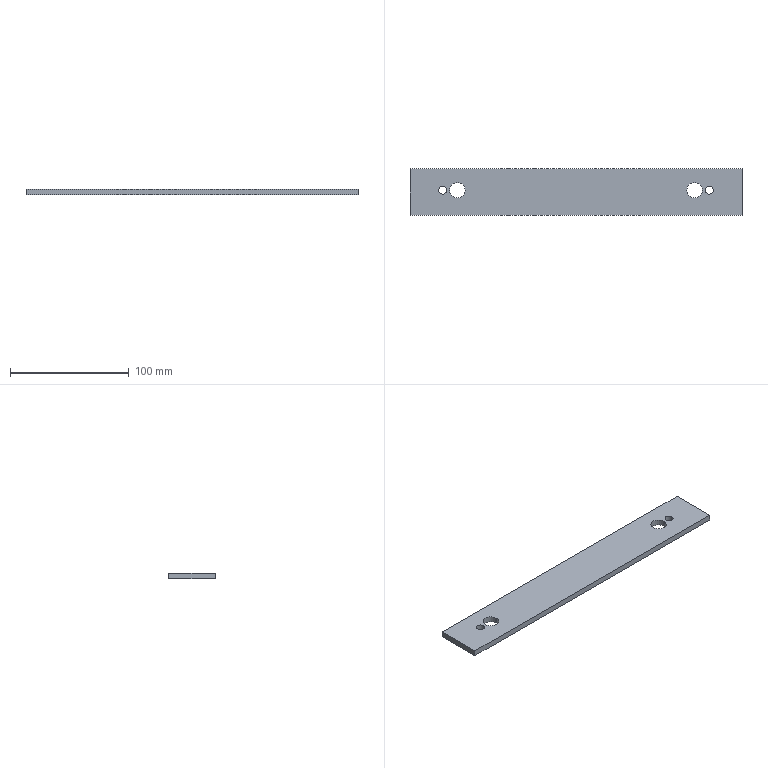Part | STEP file | 44-02-08 Ear Forming Plate A | 1 solid | 14 faces | box 280 x 39 x 5 mm | volume 52910 mm3 | cylinder 8 | plane 6 | commonest cylinder face diameters 6.8 x4 13 x4
STEP:
#1=CARTESIAN_POINT('',(0.,0.,0.));
#2=DIRECTION('',(0.,0.,1.));
#3=DIRECTION('',(1.,0.,0.));
#4=AXIS2_PLACEMENT_3D('',#1,#2,#3);
#5=CARTESIAN_POINT('',(109.1,0.,2.5));
#6=VERTEX_POINT('',#5);
#7=CARTESIAN_POINT('',(109.1,0.,-2.5));
#8=VERTEX_POINT('',#7);
#9=CARTESIAN_POINT('',(109.1,0.,-2.5));
#10=DIRECTION('',(0.,0.,-1.));
#11=VECTOR('',#10,1.);
#12=LINE('',#9,#11);
#13=CARTESIAN_POINT('',(112.5,0.,-2.5));
#14=DIRECTION('',(0.,0.,-1.));
#15=DIRECTION('',(-1.,0.,0.));
#16=AXIS2_PLACEMENT_3D('',#13,#14,#15);
#17=CYLINDRICAL_SURFACE('',#16,3.4);
#18=CARTESIAN_POINT('',(6.283,0.));
#19=DIRECTION('',(0.,1.));
#20=VECTOR('',#19,1.);
#21=LINE('',#18,#20);
#22=(GEOMETRIC_REPRESENTATION_CONTEXT(2)PARAMETRIC_REPRESENTATION_CONTEXT()REPRESENTATION_CONTEXT('',''));
#23=DEFINITIONAL_REPRESENTATION('',(#21),#22);
#24=PCURVE('',#17,#23);
#25=CARTESIAN_POINT('',(112.5,0.,-2.5));
#26=DIRECTION('',(0.,0.,-1.));
#27=DIRECTION('',(-1.,0.,0.));
#28=AXIS2_PLACEMENT_3D('',#25,#26,#27);
#29=CYLINDRICAL_SURFACE('',#28,3.4);
#30=CARTESIAN_POINT('',(0.,0.));
#31=DIRECTION('',(0.,1.));
#32=VECTOR('',#31,1.);
#33=LINE('',#30,#32);
#34=(GEOMETRIC_REPRESENTATION_CONTEXT(2)PARAMETRIC_REPRESENTATION_CONTEXT()REPRESENTATION_CONTEXT('',''));
#35=DEFINITIONAL_REPRESENTATION('',(#33),#34);
#36=PCURVE('',#29,#35);
#37=SURFACE_CURVE('',#12,(#24,#36),.PCURVE_S1.);
#38=EDGE_CURVE('',#6,#8,#37,.T.);
#39=ORIENTED_EDGE('',*,*,#38,.T.);
#40=CARTESIAN_POINT('',(115.9,0.,-2.5));
#41=VERTEX_POINT('',#40);
#42=CARTESIAN_POINT('',(112.5,0.,-2.5));
#43=DIRECTION('',(0.,0.,-1.));
#44=DIRECTION('',(-1.,0.,0.));
#45=AXIS2_PLACEMENT_3D('',#42,#43,#44);
#46=CIRCLE('',#45,3.4);
#47=CARTESIAN_POINT('',(0.,0.));
#48=DIRECTION('',(1.,0.));
#49=VECTOR('',#48,1.);
#50=LINE('',#47,#49);
#51=(GEOMETRIC_REPRESENTATION_CONTEXT(2)PARAMETRIC_REPRESENTATION_CONTEXT()REPRESENTATION_CONTEXT('',''));
#52=DEFINITIONAL_REPRESENTATION('',(#50),#51);
#53=PCURVE('',#17,#52);
#54=CARTESIAN_POINT('',(140.,-18.,-2.5));
#55=DIRECTION('',(0.,0.,1.));
#56=DIRECTION('',(1.,0.,0.));
#57=AXIS2_PLACEMENT_3D('',#54,#55,#56);
#58=PLANE('',#57);
#59=CARTESIAN_POINT('',(-30.9,18.));
#60=CARTESIAN_POINT('',(-30.9,23.889));
#61=CARTESIAN_POINT('',(-25.8,20.944));
#62=CARTESIAN_POINT('',(-20.7,18.));
#63=CARTESIAN_POINT('',(-25.8,15.056));
#64=CARTESIAN_POINT('',(-30.9,12.111));
#65=CARTESIAN_POINT('',(-30.9,18.));
#66=(BOUNDED_CURVE()B_SPLINE_CURVE(2,(#59,#60,#61,#62,#63,#64,#65),.UNSPECIFIED.,.T.,.F.)B_SPLINE_CURVE_WITH_KNOTS((1,2,2,2,2,1),(-2.094,0.,2.094,4.189,6.283,8.378),.UNSPECIFIED.)CURVE()GEOMETRIC_REPRESENTATION_ITEM()RATIONAL_B_SPLINE_CURVE((1.,0.5,1.,0.5,1.,0.5,1.))REPRESENTATION_ITEM(''));
#67=(GEOMETRIC_REPRESENTATION_CONTEXT(2)PARAMETRIC_REPRESENTATION_CONTEXT()REPRESENTATION_CONTEXT('',''));
#68=DEFINITIONAL_REPRESENTATION('',(#66),#67);
#69=PCURVE('',#58,#68);
#70=SURFACE_CURVE('',#46,(#53,#69),.PCURVE_S1.);
#71=EDGE_CURVE('',#41,#8,#70,.T.);
#72=ORIENTED_EDGE('',*,*,#71,.F.);
#73=CARTESIAN_POINT('',(115.9,0.,2.5));
#74=VERTEX_POINT('',#73);
#75=CARTESIAN_POINT('',(115.9,0.,-2.5));
#76=DIRECTION('',(0.,0.,-1.));
#77=VECTOR('',#76,1.);
#78=LINE('',#75,#77);
#79=CARTESIAN_POINT('',(3.142,0.));
#80=DIRECTION('',(0.,1.));
#81=VECTOR('',#80,1.);
#82=LINE('',#79,#81);
#83=(GEOMETRIC_REPRESENTATION_CONTEXT(2)PARAMETRIC_REPRESENTATION_CONTEXT()REPRESENTATION_CONTEXT('',''));
#84=DEFINITIONAL_REPRESENTATION('',(#82),#83);
#85=PCURVE('',#17,#84);
#86=CARTESIAN_POINT('',(3.142,0.));
#87=DIRECTION('',(0.,1.));
#88=VECTOR('',#87,1.);
#89=LINE('',#86,#88);
#90=(GEOMETRIC_REPRESENTATION_CONTEXT(2)PARAMETRIC_REPRESENTATION_CONTEXT()REPRESENTATION_CONTEXT('',''));
#91=DEFINITIONAL_REPRESENTATION('',(#89),#90);
#92=PCURVE('',#29,#91);
#93=SURFACE_CURVE('',#78,(#85,#92),.PCURVE_S1.);
#94=EDGE_CURVE('',#74,#41,#93,.T.);
#95=ORIENTED_EDGE('',*,*,#94,.F.);
#96=CARTESIAN_POINT('',(112.5,0.,2.5));
#97=DIRECTION('',(0.,0.,-1.));
#98=DIRECTION('',(-1.,0.,0.));
#99=AXIS2_PLACEMENT_3D('',#96,#97,#98);
#100=CIRCLE('',#99,3.4);
#101=CARTESIAN_POINT('',(0.,-5.));
#102=DIRECTION('',(1.,0.));
#103=VECTOR('',#102,1.);
#104=LINE('',#101,#103);
#105=(GEOMETRIC_REPRESENTATION_CONTEXT(2)PARAMETRIC_REPRESENTATION_CONTEXT()REPRESENTATION_CONTEXT('',''));
#106=DEFINITIONAL_REPRESENTATION('',(#104),#105);
#107=PCURVE('',#17,#106);
#108=CARTESIAN_POINT('',(140.,-18.,2.5));
#109=DIRECTION('',(0.,0.,1.));
#110=DIRECTION('',(1.,0.,0.));
#111=AXIS2_PLACEMENT_3D('',#108,#109,#110);
#112=PLANE('',#111);
#113=CARTESIAN_POINT('',(-30.9,18.));
#114=CARTESIAN_POINT('',(-30.9,23.889));
#115=CARTESIAN_POINT('',(-25.8,20.944));
#116=CARTESIAN_POINT('',(-20.7,18.));
#117=CARTESIAN_POINT('',(-25.8,15.056));
#118=CARTESIAN_POINT('',(-30.9,12.111));
#119=CARTESIAN_POINT('',(-30.9,18.));
#120=(BOUNDED_CURVE()B_SPLINE_CURVE(2,(#113,#114,#115,#116,#117,#118,#119),.UNSPECIFIED.,.T.,.F.)B_SPLINE_CURVE_WITH_KNOTS((1,2,2,2,2,1),(-2.094,0.,2.094,4.189,6.283,8.378),.UNSPECIFIED.)CURVE()GEOMETRIC_REPRESENTATION_ITEM()RATIONAL_B_SPLINE_CURVE((1.,0.5,1.,0.5,1.,0.5,1.))REPRESENTATION_ITEM(''));
#121=(GEOMETRIC_REPRESENTATION_CONTEXT(2)PARAMETRIC_REPRESENTATION_CONTEXT()REPRESENTATION_CONTEXT('',''));
#122=DEFINITIONAL_REPRESENTATION('',(#120),#121);
#123=PCURVE('',#112,#122);
#124=SURFACE_CURVE('',#100,(#107,#123),.PCURVE_S1.);
#125=EDGE_CURVE('',#74,#6,#124,.T.);
#126=ORIENTED_EDGE('',*,*,#125,.T.);
#127=EDGE_LOOP('',(#39,#72,#95,#126));
#128=FACE_BOUND('',#127,.F.);
#129=ADVANCED_FACE('',(#128),#17,.F.);
#130=CARTESIAN_POINT('',(-115.9,0.,2.5));
#131=VERTEX_POINT('',#130);
#132=CARTESIAN_POINT('',(-115.9,0.,-2.5));
#133=VERTEX_POINT('',#132);
#134=CARTESIAN_POINT('',(-115.9,0.,-2.5));
#135=DIRECTION('',(0.,0.,-1.));
#136=VECTOR('',#135,1.);
#137=LINE('',#134,#136);
#138=CARTESIAN_POINT('',(-112.5,0.,-2.5));
#139=DIRECTION('',(0.,0.,-1.));
#140=DIRECTION('',(-1.,0.,0.));
#141=AXIS2_PLACEMENT_3D('',#138,#139,#140);
#142=CYLINDRICAL_SURFACE('',#141,3.4);
#143=CARTESIAN_POINT('',(6.283,0.));
#144=DIRECTION('',(0.,1.));
#145=VECTOR('',#144,1.);
#146=LINE('',#143,#145);
#147=(GEOMETRIC_REPRESENTATION_CONTEXT(2)PARAMETRIC_REPRESENTATION_CONTEXT()REPRESENTATION_CONTEXT('',''));
#148=DEFINITIONAL_REPRESENTATION('',(#146),#147);
#149=PCURVE('',#142,#148);
#150=CARTESIAN_POINT('',(-112.5,0.,-2.5));
#151=DIRECTION('',(0.,0.,-1.));
#152=DIRECTION('',(-1.,0.,0.));
#153=AXIS2_PLACEMENT_3D('',#150,#151,#152);
#154=CYLINDRICAL_SURFACE('',#153,3.4);
#155=CARTESIAN_POINT('',(0.,0.));
#156=DIRECTION('',(0.,1.));
#157=VECTOR('',#156,1.);
#158=LINE('',#155,#157);
#159=(GEOMETRIC_REPRESENTATION_CONTEXT(2)PARAMETRIC_REPRESENTATION_CONTEXT()REPRESENTATION_CONTEXT('',''));
#160=DEFINITIONAL_REPRESENTATION('',(#158),#159);
#161=PCURVE('',#154,#160);
#162=SURFACE_CURVE('',#137,(#149,#161),.PCURVE_S1.);
#163=EDGE_CURVE('',#131,#133,#162,.T.);
#164=ORIENTED_EDGE('',*,*,#163,.T.);
#165=CARTESIAN_POINT('',(-109.1,0.,-2.5));
#166=VERTEX_POINT('',#165);
#167=CARTESIAN_POINT('',(-112.5,0.,-2.5));
#168=DIRECTION('',(0.,0.,-1.));
#169=DIRECTION('',(-1.,0.,0.));
#170=AXIS2_PLACEMENT_3D('',#167,#168,#169);
#171=CIRCLE('',#170,3.4);
#172=CARTESIAN_POINT('',(0.,0.));
#173=DIRECTION('',(1.,0.));
#174=VECTOR('',#173,1.);
#175=LINE('',#172,#174);
#176=(GEOMETRIC_REPRESENTATION_CONTEXT(2)PARAMETRIC_REPRESENTATION_CONTEXT()REPRESENTATION_CONTEXT('',''));
#177=DEFINITIONAL_REPRESENTATION('',(#175),#176);
#178=PCURVE('',#142,#177);
#179=CARTESIAN_POINT('',(-255.9,18.));
#180=CARTESIAN_POINT('',(-255.9,23.889));
#181=CARTESIAN_POINT('',(-250.8,20.944));
#182=CARTESIAN_POINT('',(-245.7,18.));
#183=CARTESIAN_POINT('',(-250.8,15.056));
#184=CARTESIAN_POINT('',(-255.9,12.111));
#185=CARTESIAN_POINT('',(-255.9,18.));
#186=(BOUNDED_CURVE()B_SPLINE_CURVE(2,(#179,#180,#181,#182,#183,#184,#185),.UNSPECIFIED.,.T.,.F.)B_SPLINE_CURVE_WITH_KNOTS((1,2,2,2,2,1),(-2.094,0.,2.094,4.189,6.283,8.378),.UNSPECIFIED.)CURVE()GEOMETRIC_REPRESENTATION_ITEM()RATIONAL_B_SPLINE_CURVE((1.,0.5,1.,0.5,1.,0.5,1.))REPRESENTATION_ITEM(''));
#187=(GEOMETRIC_REPRESENTATION_CONTEXT(2)PARAMETRIC_REPRESENTATION_CONTEXT()REPRESENTATION_CONTEXT('',''));
#188=DEFINITIONAL_REPRESENTATION('',(#186),#187);
#189=PCURVE('',#58,#188);
#190=SURFACE_CURVE('',#171,(#178,#189),.PCURVE_S1.);
#191=EDGE_CURVE('',#166,#133,#190,.T.);
#192=ORIENTED_EDGE('',*,*,#191,.F.);
#193=CARTESIAN_POINT('',(-109.1,0.,2.5));
#194=VERTEX_POINT('',#193);
#195=CARTESIAN_POINT('',(-109.1,0.,-2.5));
#196=DIRECTION('',(0.,0.,-1.));
#197=VECTOR('',#196,1.);
#198=LINE('',#195,#197);
#199=CARTESIAN_POINT('',(3.142,0.));
#200=DIRECTION('',(0.,1.));
#201=VECTOR('',#200,1.);
#202=LINE('',#199,#201);
#203=(GEOMETRIC_REPRESENTATION_CONTEXT(2)PARAMETRIC_REPRESENTATION_CONTEXT()REPRESENTATION_CONTEXT('',''));
#204=DEFINITIONAL_REPRESENTATION('',(#202),#203);
#205=PCURVE('',#142,#204);
#206=CARTESIAN_POINT('',(3.142,0.));
#207=DIRECTION('',(0.,1.));
#208=VECTOR('',#207,1.);
#209=LINE('',#206,#208);
#210=(GEOMETRIC_REPRESENTATION_CONTEXT(2)PARAMETRIC_REPRESENTATION_CONTEXT()REPRESENTATION_CONTEXT('',''));
#211=DEFINITIONAL_REPRESENTATION('',(#209),#210);
#212=PCURVE('',#154,#211);
#213=SURFACE_CURVE('',#198,(#205,#212),.PCURVE_S1.);
#214=EDGE_CURVE('',#194,#166,#213,.T.);
#215=ORIENTED_EDGE('',*,*,#214,.F.);
#216=CARTESIAN_POINT('',(-112.5,0.,2.5));
#217=DIRECTION('',(0.,0.,-1.));
#218=DIRECTION('',(-1.,0.,0.));
#219=AXIS2_PLACEMENT_3D('',#216,#217,#218);
#220=CIRCLE('',#219,3.4);
#221=CARTESIAN_POINT('',(0.,-5.));
#222=DIRECTION('',(1.,0.));
#223=VECTOR('',#222,1.);
#224=LINE('',#221,#223);
#225=(GEOMETRIC_REPRESENTATION_CONTEXT(2)PARAMETRIC_REPRESENTATION_CONTEXT()REPRESENTATION_CONTEXT('',''));
#226=DEFINITIONAL_REPRESENTATION('',(#224),#225);
#227=PCURVE('',#142,#226);
#228=CARTESIAN_POINT('',(-255.9,18.));
#229=CARTESIAN_POINT('',(-255.9,23.889));
#230=CARTESIAN_POINT('',(-250.8,20.944));
#231=CARTESIAN_POINT('',(-245.7,18.));
#232=CARTESIAN_POINT('',(-250.8,15.056));
#233=CARTESIAN_POINT('',(-255.9,12.111));
#234=CARTESIAN_POINT('',(-255.9,18.));
#235=(BOUNDED_CURVE()B_SPLINE_CURVE(2,(#228,#229,#230,#231,#232,#233,#234),.UNSPECIFIED.,.T.,.F.)B_SPLINE_CURVE_WITH_KNOTS((1,2,2,2,2,1),(-2.094,0.,2.094,4.189,6.283,8.378),.UNSPECIFIED.)CURVE()GEOMETRIC_REPRESENTATION_ITEM()RATIONAL_B_SPLINE_CURVE((1.,0.5,1.,0.5,1.,0.5,1.))REPRESENTATION_ITEM(''));
#236=(GEOMETRIC_REPRESENTATION_CONTEXT(2)PARAMETRIC_REPRESENTATION_CONTEXT()REPRESENTATION_CONTEXT('',''));
#237=DEFINITIONAL_REPRESENTATION('',(#235),#236);
#238=PCURVE('',#112,#237);
#239=SURFACE_CURVE('',#220,(#227,#238),.PCURVE_S1.);
#240=EDGE_CURVE('',#194,#131,#239,.T.);
#241=ORIENTED_EDGE('',*,*,#240,.T.);
#242=EDGE_LOOP('',(#164,#192,#215,#241));
#243=FACE_BOUND('',#242,.F.);
#244=ADVANCED_FACE('',(#243),#142,.F.);
#245=CARTESIAN_POINT('',(106.5,0.,-2.5));
#246=VERTEX_POINT('',#245);
#247=CARTESIAN_POINT('',(106.5,0.,2.5));
#248=VERTEX_POINT('',#247);
#249=CARTESIAN_POINT('',(106.5,0.,-2.5));
#250=DIRECTION('',(0.,0.,1.));
#251=VECTOR('',#250,1.);
#252=LINE('',#249,#251);
#253=CARTESIAN_POINT('',(100.,0.,-2.5));
#254=DIRECTION('',(0.,0.,1.));
#255=DIRECTION('',(1.,0.,0.));
#256=AXIS2_PLACEMENT_3D('',#253,#254,#255);
#257=CYLINDRICAL_SURFACE('',#256,6.5);
#258=CARTESIAN_POINT('',(6.283,0.));
#259=DIRECTION('',(0.,1.));
#260=VECTOR('',#259,1.);
#261=LINE('',#258,#260);
#262=(GEOMETRIC_REPRESENTATION_CONTEXT(2)PARAMETRIC_REPRESENTATION_CONTEXT()REPRESENTATION_CONTEXT('',''));
#263=DEFINITIONAL_REPRESENTATION('',(#261),#262);
#264=PCURVE('',#257,#263);
#265=CARTESIAN_POINT('',(100.,0.,-2.5));
#266=DIRECTION('',(0.,0.,1.));
#267=DIRECTION('',(1.,0.,0.));
#268=AXIS2_PLACEMENT_3D('',#265,#266,#267);
#269=CYLINDRICAL_SURFACE('',#268,6.5);
#270=CARTESIAN_POINT('',(0.,0.));
#271=DIRECTION('',(0.,1.));
#272=VECTOR('',#271,1.);
#273=LINE('',#270,#272);
#274=(GEOMETRIC_REPRESENTATION_CONTEXT(2)PARAMETRIC_REPRESENTATION_CONTEXT()REPRESENTATION_CONTEXT('',''));
#275=DEFINITIONAL_REPRESENTATION('',(#273),#274);
#276=PCURVE('',#269,#275);
#277=SURFACE_CURVE('',#252,(#264,#276),.PCURVE_S1.);
#278=EDGE_CURVE('',#246,#248,#277,.T.);
#279=ORIENTED_EDGE('',*,*,#278,.T.);
#280=CARTESIAN_POINT('',(93.5,0.,2.5));
#281=VERTEX_POINT('',#280);
#282=CARTESIAN_POINT('',(100.,0.,2.5));
#283=DIRECTION('',(0.,0.,1.));
#284=DIRECTION('',(1.,0.,0.));
#285=AXIS2_PLACEMENT_3D('',#282,#283,#284);
#286=CIRCLE('',#285,6.5);
#287=CARTESIAN_POINT('',(0.,5.));
#288=DIRECTION('',(1.,0.));
#289=VECTOR('',#288,1.);
#290=LINE('',#287,#289);
#291=(GEOMETRIC_REPRESENTATION_CONTEXT(2)PARAMETRIC_REPRESENTATION_CONTEXT()REPRESENTATION_CONTEXT('',''));
#292=DEFINITIONAL_REPRESENTATION('',(#290),#291);
#293=PCURVE('',#257,#292);
#294=CARTESIAN_POINT('',(-40.,18.));
#295=DIRECTION('',(1.,0.));
#296=AXIS2_PLACEMENT_2D('',#294,#295);
#297=CIRCLE('',#296,6.5);
#298=(GEOMETRIC_REPRESENTATION_CONTEXT(2)PARAMETRIC_REPRESENTATION_CONTEXT()REPRESENTATION_CONTEXT('',''));
#299=DEFINITIONAL_REPRESENTATION('',(#297),#298);
#300=PCURVE('',#112,#299);
#301=SURFACE_CURVE('',#286,(#293,#300),.PCURVE_S1.);
#302=EDGE_CURVE('',#281,#248,#301,.T.);
#303=ORIENTED_EDGE('',*,*,#302,.F.);
#304=CARTESIAN_POINT('',(93.5,0.,-2.5));
#305=VERTEX_POINT('',#304);
#306=CARTESIAN_POINT('',(93.5,0.,-2.5));
#307=DIRECTION('',(0.,0.,1.));
#308=VECTOR('',#307,1.);
#309=LINE('',#306,#308);
#310=CARTESIAN_POINT('',(3.142,0.));
#311=DIRECTION('',(0.,1.));
#312=VECTOR('',#311,1.);
#313=LINE('',#310,#312);
#314=(GEOMETRIC_REPRESENTATION_CONTEXT(2)PARAMETRIC_REPRESENTATION_CONTEXT()REPRESENTATION_CONTEXT('',''));
#315=DEFINITIONAL_REPRESENTATION('',(#313),#314);
#316=PCURVE('',#257,#315);
#317=CARTESIAN_POINT('',(3.142,0.));
#318=DIRECTION('',(0.,1.));
#319=VECTOR('',#318,1.);
#320=LINE('',#317,#319);
#321=(GEOMETRIC_REPRESENTATION_CONTEXT(2)PARAMETRIC_REPRESENTATION_CONTEXT()REPRESENTATION_CONTEXT('',''));
#322=DEFINITIONAL_REPRESENTATION('',(#320),#321);
#323=PCURVE('',#269,#322);
#324=SURFACE_CURVE('',#309,(#316,#323),.PCURVE_S1.);
#325=EDGE_CURVE('',#305,#281,#324,.T.);
#326=ORIENTED_EDGE('',*,*,#325,.F.);
#327=CARTESIAN_POINT('',(100.,0.,-2.5));
#328=DIRECTION('',(0.,0.,1.));
#329=DIRECTION('',(1.,0.,0.));
#330=AXIS2_PLACEMENT_3D('',#327,#328,#329);
#331=CIRCLE('',#330,6.5);
#332=CARTESIAN_POINT('',(0.,0.));
#333=DIRECTION('',(1.,0.));
#334=VECTOR('',#333,1.);
#335=LINE('',#332,#334);
#336=(GEOMETRIC_REPRESENTATION_CONTEXT(2)PARAMETRIC_REPRESENTATION_CONTEXT()REPRESENTATION_CONTEXT('',''));
#337=DEFINITIONAL_REPRESENTATION('',(#335),#336);
#338=PCURVE('',#257,#337);
#339=CARTESIAN_POINT('',(-40.,18.));
#340=DIRECTION('',(1.,0.));
#341=AXIS2_PLACEMENT_2D('',#339,#340);
#342=CIRCLE('',#341,6.5);
#343=(GEOMETRIC_REPRESENTATION_CONTEXT(2)PARAMETRIC_REPRESENTATION_CONTEXT()REPRESENTATION_CONTEXT('',''));
#344=DEFINITIONAL_REPRESENTATION('',(#342),#343);
#345=PCURVE('',#58,#344);
#346=SURFACE_CURVE('',#331,(#338,#345),.PCURVE_S1.);
#347=EDGE_CURVE('',#305,#246,#346,.T.);
#348=ORIENTED_EDGE('',*,*,#347,.T.);
#349=EDGE_LOOP('',(#279,#303,#326,#348));
#350=FACE_BOUND('',#349,.F.);
#351=ADVANCED_FACE('',(#350),#257,.F.);
#352=CARTESIAN_POINT('',(-93.5,0.,-2.5));
#353=VERTEX_POINT('',#352);
#354=CARTESIAN_POINT('',(-93.5,0.,2.5));
#355=VERTEX_POINT('',#354);
#356=CARTESIAN_POINT('',(-93.5,0.,-2.5));
#357=DIRECTION('',(0.,0.,1.));
#358=VECTOR('',#357,1.);
#359=LINE('',#356,#358);
#360=CARTESIAN_POINT('',(-100.,0.,-2.5));
#361=DIRECTION('',(0.,0.,1.));
#362=DIRECTION('',(1.,0.,0.));
#363=AXIS2_PLACEMENT_3D('',#360,#361,#362);
#364=CYLINDRICAL_SURFACE('',#363,6.5);
#365=CARTESIAN_POINT('',(6.283,0.));
#366=DIRECTION('',(0.,1.));
#367=VECTOR('',#366,1.);
#368=LINE('',#365,#367);
#369=(GEOMETRIC_REPRESENTATION_CONTEXT(2)PARAMETRIC_REPRESENTATION_CONTEXT()REPRESENTATION_CONTEXT('',''));
#370=DEFINITIONAL_REPRESENTATION('',(#368),#369);
#371=PCURVE('',#364,#370);
#372=CARTESIAN_POINT('',(-100.,0.,-2.5));
#373=DIRECTION('',(0.,0.,1.));
#374=DIRECTION('',(1.,0.,0.));
#375=AXIS2_PLACEMENT_3D('',#372,#373,#374);
#376=CYLINDRICAL_SURFACE('',#375,6.5);
#377=CARTESIAN_POINT('',(0.,0.));
#378=DIRECTION('',(0.,1.));
#379=VECTOR('',#378,1.);
#380=LINE('',#377,#379);
#381=(GEOMETRIC_REPRESENTATION_CONTEXT(2)PARAMETRIC_REPRESENTATION_CONTEXT()REPRESENTATION_CONTEXT('',''));
#382=DEFINITIONAL_REPRESENTATION('',(#380),#381);
#383=PCURVE('',#376,#382);
#384=SURFACE_CURVE('',#359,(#371,#383),.PCURVE_S1.);
#385=EDGE_CURVE('',#353,#355,#384,.T.);
#386=ORIENTED_EDGE('',*,*,#385,.T.);
#387=CARTESIAN_POINT('',(-106.5,0.,2.5));
#388=VERTEX_POINT('',#387);
#389=CARTESIAN_POINT('',(-100.,0.,2.5));
#390=DIRECTION('',(0.,0.,1.));
#391=DIRECTION('',(1.,0.,0.));
#392=AXIS2_PLACEMENT_3D('',#389,#390,#391);
#393=CIRCLE('',#392,6.5);
#394=CARTESIAN_POINT('',(0.,5.));
#395=DIRECTION('',(1.,0.));
#396=VECTOR('',#395,1.);
#397=LINE('',#394,#396);
#398=(GEOMETRIC_REPRESENTATION_CONTEXT(2)PARAMETRIC_REPRESENTATION_CONTEXT()REPRESENTATION_CONTEXT('',''));
#399=DEFINITIONAL_REPRESENTATION('',(#397),#398);
#400=PCURVE('',#364,#399);
#401=CARTESIAN_POINT('',(-240.,18.));
#402=DIRECTION('',(1.,0.));
#403=AXIS2_PLACEMENT_2D('',#401,#402);
#404=CIRCLE('',#403,6.5);
#405=(GEOMETRIC_REPRESENTATION_CONTEXT(2)PARAMETRIC_REPRESENTATION_CONTEXT()REPRESENTATION_CONTEXT('',''));
#406=DEFINITIONAL_REPRESENTATION('',(#404),#405);
#407=PCURVE('',#112,#406);
#408=SURFACE_CURVE('',#393,(#400,#407),.PCURVE_S1.);
#409=EDGE_CURVE('',#388,#355,#408,.T.);
#410=ORIENTED_EDGE('',*,*,#409,.F.);
#411=CARTESIAN_POINT('',(-106.5,0.,-2.5));
#412=VERTEX_POINT('',#411);
#413=CARTESIAN_POINT('',(-106.5,0.,-2.5));
#414=DIRECTION('',(0.,0.,1.));
#415=VECTOR('',#414,1.);
#416=LINE('',#413,#415);
#417=CARTESIAN_POINT('',(3.142,0.));
#418=DIRECTION('',(0.,1.));
#419=VECTOR('',#418,1.);
#420=LINE('',#417,#419);
#421=(GEOMETRIC_REPRESENTATION_CONTEXT(2)PARAMETRIC_REPRESENTATION_CONTEXT()REPRESENTATION_CONTEXT('',''));
#422=DEFINITIONAL_REPRESENTATION('',(#420),#421);
#423=PCURVE('',#364,#422);
#424=CARTESIAN_POINT('',(3.142,0.));
#425=DIRECTION('',(0.,1.));
#426=VECTOR('',#425,1.);
#427=LINE('',#424,#426);
#428=(GEOMETRIC_REPRESENTATION_CONTEXT(2)PARAMETRIC_REPRESENTATION_CONTEXT()REPRESENTATION_CONTEXT('',''));
#429=DEFINITIONAL_REPRESENTATION('',(#427),#428);
#430=PCURVE('',#376,#429);
#431=SURFACE_CURVE('',#416,(#423,#430),.PCURVE_S1.);
#432=EDGE_CURVE('',#412,#388,#431,.T.);
#433=ORIENTED_EDGE('',*,*,#432,.F.);
#434=CARTESIAN_POINT('',(-100.,0.,-2.5));
#435=DIRECTION('',(0.,0.,1.));
#436=DIRECTION('',(1.,0.,0.));
#437=AXIS2_PLACEMENT_3D('',#434,#435,#436);
#438=CIRCLE('',#437,6.5);
#439=CARTESIAN_POINT('',(0.,0.));
#440=DIRECTION('',(1.,0.));
#441=VECTOR('',#440,1.);
#442=LINE('',#439,#441);
#443=(GEOMETRIC_REPRESENTATION_CONTEXT(2)PARAMETRIC_REPRESENTATION_CONTEXT()REPRESENTATION_CONTEXT('',''));
#444=DEFINITIONAL_REPRESENTATION('',(#442),#443);
#445=PCURVE('',#364,#444);
#446=CARTESIAN_POINT('',(-240.,18.));
#447=DIRECTION('',(1.,0.));
#448=AXIS2_PLACEMENT_2D('',#446,#447);
#449=CIRCLE('',#448,6.5);
#450=(GEOMETRIC_REPRESENTATION_CONTEXT(2)PARAMETRIC_REPRESENTATION_CONTEXT()REPRESENTATION_CONTEXT('',''));
#451=DEFINITIONAL_REPRESENTATION('',(#449),#450);
#452=PCURVE('',#58,#451);
#453=SURFACE_CURVE('',#438,(#445,#452),.PCURVE_S1.);
#454=EDGE_CURVE('',#412,#353,#453,.T.);
#455=ORIENTED_EDGE('',*,*,#454,.T.);
#456=EDGE_LOOP('',(#386,#410,#433,#455));
#457=FACE_BOUND('',#456,.F.);
#458=ADVANCED_FACE('',(#457),#364,.F.);
#459=CARTESIAN_POINT('',(112.5,0.,2.5));
#460=DIRECTION('',(0.,0.,-1.));
#461=DIRECTION('',(-1.,0.,0.));
#462=AXIS2_PLACEMENT_3D('',#459,#460,#461);
#463=CIRCLE('',#462,3.4);
#464=CARTESIAN_POINT('',(-30.9,18.));
#465=CARTESIAN_POINT('',(-30.9,23.889));
#466=CARTESIAN_POINT('',(-25.8,20.944));
#467=CARTESIAN_POINT('',(-20.7,18.));
#468=CARTESIAN_POINT('',(-25.8,15.056));
#469=CARTESIAN_POINT('',(-30.9,12.111));
#470=CARTESIAN_POINT('',(-30.9,18.));
#471=(BOUNDED_CURVE()B_SPLINE_CURVE(2,(#464,#465,#466,#467,#468,#469,#470),.UNSPECIFIED.,.T.,.F.)B_SPLINE_CURVE_WITH_KNOTS((1,2,2,2,2,1),(-2.094,0.,2.094,4.189,6.283,8.378),.UNSPECIFIED.)CURVE()GEOMETRIC_REPRESENTATION_ITEM()RATIONAL_B_SPLINE_CURVE((1.,0.5,1.,0.5,1.,0.5,1.))REPRESENTATION_ITEM(''));
#472=(GEOMETRIC_REPRESENTATION_CONTEXT(2)PARAMETRIC_REPRESENTATION_CONTEXT()REPRESENTATION_CONTEXT('',''));
#473=DEFINITIONAL_REPRESENTATION('',(#471),#472);
#474=PCURVE('',#112,#473);
#475=CARTESIAN_POINT('',(0.,-5.));
#476=DIRECTION('',(1.,0.));
#477=VECTOR('',#476,1.);
#478=LINE('',#475,#477);
#479=(GEOMETRIC_REPRESENTATION_CONTEXT(2)PARAMETRIC_REPRESENTATION_CONTEXT()REPRESENTATION_CONTEXT('',''));
#480=DEFINITIONAL_REPRESENTATION('',(#478),#479);
#481=PCURVE('',#29,#480);
#482=SURFACE_CURVE('',#463,(#474,#481),.PCURVE_S1.);
#483=EDGE_CURVE('',#6,#74,#482,.T.);
#484=ORIENTED_EDGE('',*,*,#483,.T.);
#485=ORIENTED_EDGE('',*,*,#125,.T.);
#486=EDGE_LOOP('',(#484,#485));
#487=FACE_BOUND('',#486,.T.);
#488=CARTESIAN_POINT('',(140.,-21.,2.5));
#489=VERTEX_POINT('',#488);
#490=CARTESIAN_POINT('',(140.,18.,2.5));
#491=VERTEX_POINT('',#490);
#492=CARTESIAN_POINT('',(140.,18.,2.5));
#493=DIRECTION('',(0.,1.,0.));
#494=VECTOR('',#493,1.);
#495=LINE('',#492,#494);
#496=CARTESIAN_POINT('',(0.,36.));
#497=DIRECTION('',(0.,1.));
#498=VECTOR('',#497,1.);
#499=LINE('',#496,#498);
#500=(GEOMETRIC_REPRESENTATION_CONTEXT(2)PARAMETRIC_REPRESENTATION_CONTEXT()REPRESENTATION_CONTEXT('',''));
#501=DEFINITIONAL_REPRESENTATION('',(#499),#500);
#502=PCURVE('',#112,#501);
#503=CARTESIAN_POINT('',(140.,18.,2.5));
#504=DIRECTION('',(-1.,0.,0.));
#505=DIRECTION('',(0.,0.,1.));
#506=AXIS2_PLACEMENT_3D('',#503,#504,#505);
#507=PLANE('',#506);
#508=CARTESIAN_POINT('',(0.,0.));
#509=DIRECTION('',(0.,1.));
#510=VECTOR('',#509,1.);
#511=LINE('',#508,#510);
#512=(GEOMETRIC_REPRESENTATION_CONTEXT(2)PARAMETRIC_REPRESENTATION_CONTEXT()REPRESENTATION_CONTEXT('',''));
#513=DEFINITIONAL_REPRESENTATION('',(#511),#512);
#514=PCURVE('',#507,#513);
#515=SURFACE_CURVE('',#495,(#502,#514),.PCURVE_S1.);
#516=EDGE_CURVE('',#489,#491,#515,.T.);
#517=ORIENTED_EDGE('',*,*,#516,.T.);
#518=CARTESIAN_POINT('',(-140.,18.,2.5));
#519=VERTEX_POINT('',#518);
#520=CARTESIAN_POINT('',(-140.,18.,2.5));
#521=DIRECTION('',(-1.,0.,0.));
#522=VECTOR('',#521,1.);
#523=LINE('',#520,#522);
#524=CARTESIAN_POINT('',(-280.,36.));
#525=DIRECTION('',(-1.,0.));
#526=VECTOR('',#525,1.);
#527=LINE('',#524,#526);
#528=(GEOMETRIC_REPRESENTATION_CONTEXT(2)PARAMETRIC_REPRESENTATION_CONTEXT()REPRESENTATION_CONTEXT('',''));
#529=DEFINITIONAL_REPRESENTATION('',(#527),#528);
#530=PCURVE('',#112,#529);
#531=CARTESIAN_POINT('',(-140.,18.,2.5));
#532=DIRECTION('',(0.,-1.,0.));
#533=DIRECTION('',(0.,0.,-1.));
#534=AXIS2_PLACEMENT_3D('',#531,#532,#533);
#535=PLANE('',#534);
#536=CARTESIAN_POINT('',(0.,0.));
#537=DIRECTION('',(0.,-1.));
#538=VECTOR('',#537,1.);
#539=LINE('',#536,#538);
#540=(GEOMETRIC_REPRESENTATION_CONTEXT(2)PARAMETRIC_REPRESENTATION_CONTEXT()REPRESENTATION_CONTEXT('',''));
#541=DEFINITIONAL_REPRESENTATION('',(#539),#540);
#542=PCURVE('',#535,#541);
#543=SURFACE_CURVE('',#523,(#530,#542),.PCURVE_S1.);
#544=EDGE_CURVE('',#491,#519,#543,.T.);
#545=ORIENTED_EDGE('',*,*,#544,.T.);
#546=CARTESIAN_POINT('',(-140.,-21.,2.5));
#547=VERTEX_POINT('',#546);
#548=CARTESIAN_POINT('',(-140.,18.,2.5));
#549=DIRECTION('',(0.,-1.,0.));
#550=VECTOR('',#549,1.);
#551=LINE('',#548,#550);
#552=CARTESIAN_POINT('',(-280.,36.));
#553=DIRECTION('',(0.,-1.));
#554=VECTOR('',#553,1.);
#555=LINE('',#552,#554);
#556=(GEOMETRIC_REPRESENTATION_CONTEXT(2)PARAMETRIC_REPRESENTATION_CONTEXT()REPRESENTATION_CONTEXT('',''));
#557=DEFINITIONAL_REPRESENTATION('',(#555),#556);
#558=PCURVE('',#112,#557);
#559=CARTESIAN_POINT('',(-140.,18.,2.5));
#560=DIRECTION('',(1.,0.,0.));
#561=DIRECTION('',(0.,0.,-1.));
#562=AXIS2_PLACEMENT_3D('',#559,#560,#561);
#563=PLANE('',#562);
#564=CARTESIAN_POINT('',(0.,0.));
#565=DIRECTION('',(0.,-1.));
#566=VECTOR('',#565,1.);
#567=LINE('',#564,#566);
#568=(GEOMETRIC_REPRESENTATION_CONTEXT(2)PARAMETRIC_REPRESENTATION_CONTEXT()REPRESENTATION_CONTEXT('',''));
#569=DEFINITIONAL_REPRESENTATION('',(#567),#568);
#570=PCURVE('',#563,#569);
#571=SURFACE_CURVE('',#551,(#558,#570),.PCURVE_S1.);
#572=EDGE_CURVE('',#519,#547,#571,.T.);
#573=ORIENTED_EDGE('',*,*,#572,.T.);
#574=CARTESIAN_POINT('',(-140.,-21.,2.5));
#575=DIRECTION('',(1.,0.,0.));
#576=VECTOR('',#575,1.);
#577=LINE('',#574,#576);
#578=CARTESIAN_POINT('',(-280.,-3.));
#579=DIRECTION('',(1.,0.));
#580=VECTOR('',#579,1.);
#581=LINE('',#578,#580);
#582=(GEOMETRIC_REPRESENTATION_CONTEXT(2)PARAMETRIC_REPRESENTATION_CONTEXT()REPRESENTATION_CONTEXT('',''));
#583=DEFINITIONAL_REPRESENTATION('',(#581),#582);
#584=PCURVE('',#112,#583);
#585=CARTESIAN_POINT('',(-140.,-21.,2.5));
#586=DIRECTION('',(0.,1.,0.));
#587=DIRECTION('',(0.,0.,1.));
#588=AXIS2_PLACEMENT_3D('',#585,#586,#587);
#589=PLANE('',#588);
#590=CARTESIAN_POINT('',(0.,0.));
#591=DIRECTION('',(0.,1.));
#592=VECTOR('',#591,1.);
#593=LINE('',#590,#592);
#594=(GEOMETRIC_REPRESENTATION_CONTEXT(2)PARAMETRIC_REPRESENTATION_CONTEXT()REPRESENTATION_CONTEXT('',''));
#595=DEFINITIONAL_REPRESENTATION('',(#593),#594);
#596=PCURVE('',#589,#595);
#597=SURFACE_CURVE('',#577,(#584,#596),.PCURVE_S1.);
#598=EDGE_CURVE('',#547,#489,#597,.T.);
#599=ORIENTED_EDGE('',*,*,#598,.T.);
#600=EDGE_LOOP('',(#517,#545,#573,#599));
#601=FACE_BOUND('',#600,.T.);
#602=CARTESIAN_POINT('',(-100.,0.,2.5));
#603=DIRECTION('',(0.,0.,1.));
#604=DIRECTION('',(1.,0.,0.));
#605=AXIS2_PLACEMENT_3D('',#602,#603,#604);
#606=CIRCLE('',#605,6.5);
#607=CARTESIAN_POINT('',(-240.,18.));
#608=DIRECTION('',(1.,0.));
#609=AXIS2_PLACEMENT_2D('',#607,#608);
#610=CIRCLE('',#609,6.5);
#611=(GEOMETRIC_REPRESENTATION_CONTEXT(2)PARAMETRIC_REPRESENTATION_CONTEXT()REPRESENTATION_CONTEXT('',''));
#612=DEFINITIONAL_REPRESENTATION('',(#610),#611);
#613=PCURVE('',#112,#612);
#614=CARTESIAN_POINT('',(0.,5.));
#615=DIRECTION('',(1.,0.));
#616=VECTOR('',#615,1.);
#617=LINE('',#614,#616);
#618=(GEOMETRIC_REPRESENTATION_CONTEXT(2)PARAMETRIC_REPRESENTATION_CONTEXT()REPRESENTATION_CONTEXT('',''));
#619=DEFINITIONAL_REPRESENTATION('',(#617),#618);
#620=PCURVE('',#376,#619);
#621=SURFACE_CURVE('',#606,(#613,#620),.PCURVE_S1.);
#622=EDGE_CURVE('',#355,#388,#621,.T.);
#623=ORIENTED_EDGE('',*,*,#622,.F.);
#624=ORIENTED_EDGE('',*,*,#409,.F.);
#625=EDGE_LOOP('',(#623,#624));
#626=FACE_BOUND('',#625,.T.);
#627=CARTESIAN_POINT('',(100.,0.,2.5));
#628=DIRECTION('',(0.,0.,1.));
#629=DIRECTION('',(1.,0.,0.));
#630=AXIS2_PLACEMENT_3D('',#627,#628,#629);
#631=CIRCLE('',#630,6.5);
#632=CARTESIAN_POINT('',(-40.,18.));
#633=DIRECTION('',(1.,0.));
#634=AXIS2_PLACEMENT_2D('',#632,#633);
#635=CIRCLE('',#634,6.5);
#636=(GEOMETRIC_REPRESENTATION_CONTEXT(2)PARAMETRIC_REPRESENTATION_CONTEXT()REPRESENTATION_CONTEXT('',''));
#637=DEFINITIONAL_REPRESENTATION('',(#635),#636);
#638=PCURVE('',#112,#637);
#639=CARTESIAN_POINT('',(0.,5.));
#640=DIRECTION('',(1.,0.));
#641=VECTOR('',#640,1.);
#642=LINE('',#639,#641);
#643=(GEOMETRIC_REPRESENTATION_CONTEXT(2)PARAMETRIC_REPRESENTATION_CONTEXT()REPRESENTATION_CONTEXT('',''));
#644=DEFINITIONAL_REPRESENTATION('',(#642),#643);
#645=PCURVE('',#269,#644);
#646=SURFACE_CURVE('',#631,(#638,#645),.PCURVE_S1.);
#647=EDGE_CURVE('',#248,#281,#646,.T.);
#648=ORIENTED_EDGE('',*,*,#647,.F.);
#649=ORIENTED_EDGE('',*,*,#302,.F.);
#650=EDGE_LOOP('',(#648,#649));
#651=FACE_BOUND('',#650,.T.);
#652=CARTESIAN_POINT('',(-112.5,0.,2.5));
#653=DIRECTION('',(0.,0.,-1.));
#654=DIRECTION('',(-1.,0.,0.));
#655=AXIS2_PLACEMENT_3D('',#652,#653,#654);
#656=CIRCLE('',#655,3.4);
#657=CARTESIAN_POINT('',(-255.9,18.));
#658=CARTESIAN_POINT('',(-255.9,23.889));
#659=CARTESIAN_POINT('',(-250.8,20.944));
#660=CARTESIAN_POINT('',(-245.7,18.));
#661=CARTESIAN_POINT('',(-250.8,15.056));
#662=CARTESIAN_POINT('',(-255.9,12.111));
#663=CARTESIAN_POINT('',(-255.9,18.));
#664=(BOUNDED_CURVE()B_SPLINE_CURVE(2,(#657,#658,#659,#660,#661,#662,#663),.UNSPECIFIED.,.T.,.F.)B_SPLINE_CURVE_WITH_KNOTS((1,2,2,2,2,1),(-2.094,0.,2.094,4.189,6.283,8.378),.UNSPECIFIED.)CURVE()GEOMETRIC_REPRESENTATION_ITEM()RATIONAL_B_SPLINE_CURVE((1.,0.5,1.,0.5,1.,0.5,1.))REPRESENTATION_ITEM(''));
#665=(GEOMETRIC_REPRESENTATION_CONTEXT(2)PARAMETRIC_REPRESENTATION_CONTEXT()REPRESENTATION_CONTEXT('',''));
#666=DEFINITIONAL_REPRESENTATION('',(#664),#665);
#667=PCURVE('',#112,#666);
#668=CARTESIAN_POINT('',(0.,-5.));
#669=DIRECTION('',(1.,0.));
#670=VECTOR('',#669,1.);
#671=LINE('',#668,#670);
#672=(GEOMETRIC_REPRESENTATION_CONTEXT(2)PARAMETRIC_REPRESENTATION_CONTEXT()REPRESENTATION_CONTEXT('',''));
#673=DEFINITIONAL_REPRESENTATION('',(#671),#672);
#674=PCURVE('',#154,#673);
#675=SURFACE_CURVE('',#656,(#667,#674),.PCURVE_S1.);
#676=EDGE_CURVE('',#131,#194,#675,.T.);
#677=ORIENTED_EDGE('',*,*,#676,.T.);
#678=ORIENTED_EDGE('',*,*,#240,.T.);
#679=EDGE_LOOP('',(#677,#678));
#680=FACE_BOUND('',#679,.T.);
#681=ADVANCED_FACE('',(#487,#601,#626,#651,#680),#112,.T.);
#682=CARTESIAN_POINT('',(140.,-21.,-2.5));
#683=VERTEX_POINT('',#682);
#684=CARTESIAN_POINT('',(140.,18.,-2.5));
#685=VERTEX_POINT('',#684);
#686=CARTESIAN_POINT('',(140.,18.,-2.5));
#687=DIRECTION('',(0.,1.,0.));
#688=VECTOR('',#687,1.);
#689=LINE('',#686,#688);
#690=CARTESIAN_POINT('',(-5.,0.));
#691=DIRECTION('',(0.,1.));
#692=VECTOR('',#691,1.);
#693=LINE('',#690,#692);
#694=(GEOMETRIC_REPRESENTATION_CONTEXT(2)PARAMETRIC_REPRESENTATION_CONTEXT()REPRESENTATION_CONTEXT('',''));
#695=DEFINITIONAL_REPRESENTATION('',(#693),#694);
#696=PCURVE('',#507,#695);
#697=CARTESIAN_POINT('',(0.,36.));
#698=DIRECTION('',(0.,1.));
#699=VECTOR('',#698,1.);
#700=LINE('',#697,#699);
#701=(GEOMETRIC_REPRESENTATION_CONTEXT(2)PARAMETRIC_REPRESENTATION_CONTEXT()REPRESENTATION_CONTEXT('',''));
#702=DEFINITIONAL_REPRESENTATION('',(#700),#701);
#703=PCURVE('',#58,#702);
#704=SURFACE_CURVE('',#689,(#696,#703),.PCURVE_S1.);
#705=EDGE_CURVE('',#683,#685,#704,.T.);
#706=ORIENTED_EDGE('',*,*,#705,.T.);
#707=CARTESIAN_POINT('',(140.,18.,2.5));
#708=DIRECTION('',(0.,0.,-1.));
#709=VECTOR('',#708,1.);
#710=LINE('',#707,#709);
#711=CARTESIAN_POINT('',(0.,0.));
#712=DIRECTION('',(-1.,0.));
#713=VECTOR('',#712,1.);
#714=LINE('',#711,#713);
#715=(GEOMETRIC_REPRESENTATION_CONTEXT(2)PARAMETRIC_REPRESENTATION_CONTEXT()REPRESENTATION_CONTEXT('',''));
#716=DEFINITIONAL_REPRESENTATION('',(#714),#715);
#717=PCURVE('',#507,#716);
#718=CARTESIAN_POINT('',(0.,280.));
#719=DIRECTION('',(1.,0.));
#720=VECTOR('',#719,1.);
#721=LINE('',#718,#720);
#722=(GEOMETRIC_REPRESENTATION_CONTEXT(2)PARAMETRIC_REPRESENTATION_CONTEXT()REPRESENTATION_CONTEXT('',''));
#723=DEFINITIONAL_REPRESENTATION('',(#721),#722);
#724=PCURVE('',#535,#723);
#725=SURFACE_CURVE('',#710,(#717,#724),.PCURVE_S1.);
#726=EDGE_CURVE('',#491,#685,#725,.T.);
#727=ORIENTED_EDGE('',*,*,#726,.F.);
#728=ORIENTED_EDGE('',*,*,#516,.F.);
#729=CARTESIAN_POINT('',(140.,-21.,-2.5));
#730=DIRECTION('',(0.,0.,-1.));
#731=VECTOR('',#730,1.);
#732=LINE('',#729,#731);
#733=CARTESIAN_POINT('',(-5.,-39.));
#734=DIRECTION('',(-1.,0.));
#735=VECTOR('',#734,1.);
#736=LINE('',#733,#735);
#737=(GEOMETRIC_REPRESENTATION_CONTEXT(2)PARAMETRIC_REPRESENTATION_CONTEXT()REPRESENTATION_CONTEXT('',''));
#738=DEFINITIONAL_REPRESENTATION('',(#736),#737);
#739=PCURVE('',#507,#738);
#740=CARTESIAN_POINT('',(-5.,280.));
#741=DIRECTION('',(-1.,0.));
#742=VECTOR('',#741,1.);
#743=LINE('',#740,#742);
#744=(GEOMETRIC_REPRESENTATION_CONTEXT(2)PARAMETRIC_REPRESENTATION_CONTEXT()REPRESENTATION_CONTEXT('',''));
#745=DEFINITIONAL_REPRESENTATION('',(#743),#744);
#746=PCURVE('',#589,#745);
#747=SURFACE_CURVE('',#732,(#739,#746),.PCURVE_S1.);
#748=EDGE_CURVE('',#489,#683,#747,.T.);
#749=ORIENTED_EDGE('',*,*,#748,.T.);
#750=EDGE_LOOP('',(#706,#727,#728,#749));
#751=FACE_BOUND('',#750,.T.);
#752=ADVANCED_FACE('',(#751),#507,.F.);
#753=CARTESIAN_POINT('',(-140.,18.,-2.5));
#754=VERTEX_POINT('',#753);
#755=CARTESIAN_POINT('',(-140.,18.,-2.5));
#756=DIRECTION('',(-1.,0.,0.));
#757=VECTOR('',#756,1.);
#758=LINE('',#755,#757);
#759=CARTESIAN_POINT('',(5.,0.));
#760=DIRECTION('',(0.,-1.));
#761=VECTOR('',#760,1.);
#762=LINE('',#759,#761);
#763=(GEOMETRIC_REPRESENTATION_CONTEXT(2)PARAMETRIC_REPRESENTATION_CONTEXT()REPRESENTATION_CONTEXT('',''));
#764=DEFINITIONAL_REPRESENTATION('',(#762),#763);
#765=PCURVE('',#535,#764);
#766=CARTESIAN_POINT('',(-280.,36.));
#767=DIRECTION('',(-1.,0.));
#768=VECTOR('',#767,1.);
#769=LINE('',#766,#768);
#770=(GEOMETRIC_REPRESENTATION_CONTEXT(2)PARAMETRIC_REPRESENTATION_CONTEXT()REPRESENTATION_CONTEXT('',''));
#771=DEFINITIONAL_REPRESENTATION('',(#769),#770);
#772=PCURVE('',#58,#771);
#773=SURFACE_CURVE('',#758,(#765,#772),.PCURVE_S1.);
#774=EDGE_CURVE('',#685,#754,#773,.T.);
#775=ORIENTED_EDGE('',*,*,#774,.T.);
#776=CARTESIAN_POINT('',(-140.,18.,2.5));
#777=DIRECTION('',(0.,0.,-1.));
#778=VECTOR('',#777,1.);
#779=LINE('',#776,#778);
#780=CARTESIAN_POINT('',(0.,0.));
#781=DIRECTION('',(1.,0.));
#782=VECTOR('',#781,1.);
#783=LINE('',#780,#782);
#784=(GEOMETRIC_REPRESENTATION_CONTEXT(2)PARAMETRIC_REPRESENTATION_CONTEXT()REPRESENTATION_CONTEXT('',''));
#785=DEFINITIONAL_REPRESENTATION('',(#783),#784);
#786=PCURVE('',#535,#785);
#787=CARTESIAN_POINT('',(0.,0.));
#788=DIRECTION('',(1.,0.));
#789=VECTOR('',#788,1.);
#790=LINE('',#787,#789);
#791=(GEOMETRIC_REPRESENTATION_CONTEXT(2)PARAMETRIC_REPRESENTATION_CONTEXT()REPRESENTATION_CONTEXT('',''));
#792=DEFINITIONAL_REPRESENTATION('',(#790),#791);
#793=PCURVE('',#563,#792);
#794=SURFACE_CURVE('',#779,(#786,#793),.PCURVE_S1.);
#795=EDGE_CURVE('',#519,#754,#794,.T.);
#796=ORIENTED_EDGE('',*,*,#795,.F.);
#797=ORIENTED_EDGE('',*,*,#544,.F.);
#798=ORIENTED_EDGE('',*,*,#726,.T.);
#799=EDGE_LOOP('',(#775,#796,#797,#798));
#800=FACE_BOUND('',#799,.T.);
#801=ADVANCED_FACE('',(#800),#535,.F.);
#802=CARTESIAN_POINT('',(-140.,-21.,-2.5));
#803=VERTEX_POINT('',#802);
#804=CARTESIAN_POINT('',(-140.,18.,-2.5));
#805=DIRECTION('',(0.,-1.,0.));
#806=VECTOR('',#805,1.);
#807=LINE('',#804,#806);
#808=CARTESIAN_POINT('',(5.,0.));
#809=DIRECTION('',(0.,-1.));
#810=VECTOR('',#809,1.);
#811=LINE('',#808,#810);
#812=(GEOMETRIC_REPRESENTATION_CONTEXT(2)PARAMETRIC_REPRESENTATION_CONTEXT()REPRESENTATION_CONTEXT('',''));
#813=DEFINITIONAL_REPRESENTATION('',(#811),#812);
#814=PCURVE('',#563,#813);
#815=CARTESIAN_POINT('',(-280.,36.));
#816=DIRECTION('',(0.,-1.));
#817=VECTOR('',#816,1.);
#818=LINE('',#815,#817);
#819=(GEOMETRIC_REPRESENTATION_CONTEXT(2)PARAMETRIC_REPRESENTATION_CONTEXT()REPRESENTATION_CONTEXT('',''));
#820=DEFINITIONAL_REPRESENTATION('',(#818),#819);
#821=PCURVE('',#58,#820);
#822=SURFACE_CURVE('',#807,(#814,#821),.PCURVE_S1.);
#823=EDGE_CURVE('',#754,#803,#822,.T.);
#824=ORIENTED_EDGE('',*,*,#823,.T.);
#825=CARTESIAN_POINT('',(-140.,-21.,-2.5));
#826=DIRECTION('',(0.,0.,1.));
#827=VECTOR('',#826,1.);
#828=LINE('',#825,#827);
#829=CARTESIAN_POINT('',(5.,-39.));
#830=DIRECTION('',(-1.,0.));
#831=VECTOR('',#830,1.);
#832=LINE('',#829,#831);
#833=(GEOMETRIC_REPRESENTATION_CONTEXT(2)PARAMETRIC_REPRESENTATION_CONTEXT()REPRESENTATION_CONTEXT('',''));
#834=DEFINITIONAL_REPRESENTATION('',(#832),#833);
#835=PCURVE('',#563,#834);
#836=CARTESIAN_POINT('',(-5.,0.));
#837=DIRECTION('',(1.,0.));
#838=VECTOR('',#837,1.);
#839=LINE('',#836,#838);
#840=(GEOMETRIC_REPRESENTATION_CONTEXT(2)PARAMETRIC_REPRESENTATION_CONTEXT()REPRESENTATION_CONTEXT('',''));
#841=DEFINITIONAL_REPRESENTATION('',(#839),#840);
#842=PCURVE('',#589,#841);
#843=SURFACE_CURVE('',#828,(#835,#842),.PCURVE_S1.);
#844=EDGE_CURVE('',#803,#547,#843,.T.);
#845=ORIENTED_EDGE('',*,*,#844,.T.);
#846=ORIENTED_EDGE('',*,*,#572,.F.);
#847=ORIENTED_EDGE('',*,*,#795,.T.);
#848=EDGE_LOOP('',(#824,#845,#846,#847));
#849=FACE_BOUND('',#848,.T.);
#850=ADVANCED_FACE('',(#849),#563,.F.);
#851=CARTESIAN_POINT('',(112.5,0.,-2.5));
#852=DIRECTION('',(0.,0.,-1.));
#853=DIRECTION('',(-1.,0.,0.));
#854=AXIS2_PLACEMENT_3D('',#851,#852,#853);
#855=CIRCLE('',#854,3.4);
#856=CARTESIAN_POINT('',(-30.9,18.));
#857=CARTESIAN_POINT('',(-30.9,23.889));
#858=CARTESIAN_POINT('',(-25.8,20.944));
#859=CARTESIAN_POINT('',(-20.7,18.));
#860=CARTESIAN_POINT('',(-25.8,15.056));
#861=CARTESIAN_POINT('',(-30.9,12.111));
#862=CARTESIAN_POINT('',(-30.9,18.));
#863=(BOUNDED_CURVE()B_SPLINE_CURVE(2,(#856,#857,#858,#859,#860,#861,#862),.UNSPECIFIED.,.T.,.F.)B_SPLINE_CURVE_WITH_KNOTS((1,2,2,2,2,1),(-2.094,0.,2.094,4.189,6.283,8.378),.UNSPECIFIED.)CURVE()GEOMETRIC_REPRESENTATION_ITEM()RATIONAL_B_SPLINE_CURVE((1.,0.5,1.,0.5,1.,0.5,1.))REPRESENTATION_ITEM(''));
#864=(GEOMETRIC_REPRESENTATION_CONTEXT(2)PARAMETRIC_REPRESENTATION_CONTEXT()REPRESENTATION_CONTEXT('',''));
#865=DEFINITIONAL_REPRESENTATION('',(#863),#864);
#866=PCURVE('',#58,#865);
#867=CARTESIAN_POINT('',(0.,0.));
#868=DIRECTION('',(1.,0.));
#869=VECTOR('',#868,1.);
#870=LINE('',#867,#869);
#871=(GEOMETRIC_REPRESENTATION_CONTEXT(2)PARAMETRIC_REPRESENTATION_CONTEXT()REPRESENTATION_CONTEXT('',''));
#872=DEFINITIONAL_REPRESENTATION('',(#870),#871);
#873=PCURVE('',#29,#872);
#874=SURFACE_CURVE('',#855,(#866,#873),.PCURVE_S1.);
#875=EDGE_CURVE('',#8,#41,#874,.T.);
#876=ORIENTED_EDGE('',*,*,#875,.F.);
#877=ORIENTED_EDGE('',*,*,#71,.F.);
#878=EDGE_LOOP('',(#876,#877));
#879=FACE_BOUND('',#878,.T.);
#880=CARTESIAN_POINT('',(-112.5,0.,-2.5));
#881=DIRECTION('',(0.,0.,-1.));
#882=DIRECTION('',(-1.,0.,0.));
#883=AXIS2_PLACEMENT_3D('',#880,#881,#882);
#884=CIRCLE('',#883,3.4);
#885=CARTESIAN_POINT('',(-255.9,18.));
#886=CARTESIAN_POINT('',(-255.9,23.889));
#887=CARTESIAN_POINT('',(-250.8,20.944));
#888=CARTESIAN_POINT('',(-245.7,18.));
#889=CARTESIAN_POINT('',(-250.8,15.056));
#890=CARTESIAN_POINT('',(-255.9,12.111));
#891=CARTESIAN_POINT('',(-255.9,18.));
#892=(BOUNDED_CURVE()B_SPLINE_CURVE(2,(#885,#886,#887,#888,#889,#890,#891),.UNSPECIFIED.,.T.,.F.)B_SPLINE_CURVE_WITH_KNOTS((1,2,2,2,2,1),(-2.094,0.,2.094,4.189,6.283,8.378),.UNSPECIFIED.)CURVE()GEOMETRIC_REPRESENTATION_ITEM()RATIONAL_B_SPLINE_CURVE((1.,0.5,1.,0.5,1.,0.5,1.))REPRESENTATION_ITEM(''));
#893=(GEOMETRIC_REPRESENTATION_CONTEXT(2)PARAMETRIC_REPRESENTATION_CONTEXT()REPRESENTATION_CONTEXT('',''));
#894=DEFINITIONAL_REPRESENTATION('',(#892),#893);
#895=PCURVE('',#58,#894);
#896=CARTESIAN_POINT('',(0.,0.));
#897=DIRECTION('',(1.,0.));
#898=VECTOR('',#897,1.);
#899=LINE('',#896,#898);
#900=(GEOMETRIC_REPRESENTATION_CONTEXT(2)PARAMETRIC_REPRESENTATION_CONTEXT()REPRESENTATION_CONTEXT('',''));
#901=DEFINITIONAL_REPRESENTATION('',(#899),#900);
#902=PCURVE('',#154,#901);
#903=SURFACE_CURVE('',#884,(#895,#902),.PCURVE_S1.);
#904=EDGE_CURVE('',#133,#166,#903,.T.);
#905=ORIENTED_EDGE('',*,*,#904,.F.);
#906=ORIENTED_EDGE('',*,*,#191,.F.);
#907=EDGE_LOOP('',(#905,#906));
#908=FACE_BOUND('',#907,.T.);
#909=CARTESIAN_POINT('',(100.,0.,-2.5));
#910=DIRECTION('',(0.,0.,1.));
#911=DIRECTION('',(1.,0.,0.));
#912=AXIS2_PLACEMENT_3D('',#909,#910,#911);
#913=CIRCLE('',#912,6.5);
#914=CARTESIAN_POINT('',(-40.,18.));
#915=DIRECTION('',(1.,0.));
#916=AXIS2_PLACEMENT_2D('',#914,#915);
#917=CIRCLE('',#916,6.5);
#918=(GEOMETRIC_REPRESENTATION_CONTEXT(2)PARAMETRIC_REPRESENTATION_CONTEXT()REPRESENTATION_CONTEXT('',''));
#919=DEFINITIONAL_REPRESENTATION('',(#917),#918);
#920=PCURVE('',#58,#919);
#921=CARTESIAN_POINT('',(0.,0.));
#922=DIRECTION('',(1.,0.));
#923=VECTOR('',#922,1.);
#924=LINE('',#921,#923);
#925=(GEOMETRIC_REPRESENTATION_CONTEXT(2)PARAMETRIC_REPRESENTATION_CONTEXT()REPRESENTATION_CONTEXT('',''));
#926=DEFINITIONAL_REPRESENTATION('',(#924),#925);
#927=PCURVE('',#269,#926);
#928=SURFACE_CURVE('',#913,(#920,#927),.PCURVE_S1.);
#929=EDGE_CURVE('',#246,#305,#928,.T.);
#930=ORIENTED_EDGE('',*,*,#929,.T.);
#931=ORIENTED_EDGE('',*,*,#347,.T.);
#932=EDGE_LOOP('',(#930,#931));
#933=FACE_BOUND('',#932,.T.);
#934=CARTESIAN_POINT('',(-100.,0.,-2.5));
#935=DIRECTION('',(0.,0.,1.));
#936=DIRECTION('',(1.,0.,0.));
#937=AXIS2_PLACEMENT_3D('',#934,#935,#936);
#938=CIRCLE('',#937,6.5);
#939=CARTESIAN_POINT('',(-240.,18.));
#940=DIRECTION('',(1.,0.));
#941=AXIS2_PLACEMENT_2D('',#939,#940);
#942=CIRCLE('',#941,6.5);
#943=(GEOMETRIC_REPRESENTATION_CONTEXT(2)PARAMETRIC_REPRESENTATION_CONTEXT()REPRESENTATION_CONTEXT('',''));
#944=DEFINITIONAL_REPRESENTATION('',(#942),#943);
#945=PCURVE('',#58,#944);
#946=CARTESIAN_POINT('',(0.,0.));
#947=DIRECTION('',(1.,0.));
#948=VECTOR('',#947,1.);
#949=LINE('',#946,#948);
#950=(GEOMETRIC_REPRESENTATION_CONTEXT(2)PARAMETRIC_REPRESENTATION_CONTEXT()REPRESENTATION_CONTEXT('',''));
#951=DEFINITIONAL_REPRESENTATION('',(#949),#950);
#952=PCURVE('',#376,#951);
#953=SURFACE_CURVE('',#938,(#945,#952),.PCURVE_S1.);
#954=EDGE_CURVE('',#353,#412,#953,.T.);
#955=ORIENTED_EDGE('',*,*,#954,.T.);
#956=ORIENTED_EDGE('',*,*,#454,.T.);
#957=EDGE_LOOP('',(#955,#956));
#958=FACE_BOUND('',#957,.T.);
#959=ORIENTED_EDGE('',*,*,#705,.F.);
#960=CARTESIAN_POINT('',(-140.,-21.,-2.5));
#961=DIRECTION('',(-1.,0.,0.));
#962=VECTOR('',#961,1.);
#963=LINE('',#960,#962);
#964=CARTESIAN_POINT('',(-280.,-3.));
#965=DIRECTION('',(-1.,0.));
#966=VECTOR('',#965,1.);
#967=LINE('',#964,#966);
#968=(GEOMETRIC_REPRESENTATION_CONTEXT(2)PARAMETRIC_REPRESENTATION_CONTEXT()REPRESENTATION_CONTEXT('',''));
#969=DEFINITIONAL_REPRESENTATION('',(#967),#968);
#970=PCURVE('',#58,#969);
#971=CARTESIAN_POINT('',(-5.,0.));
#972=DIRECTION('',(0.,-1.));
#973=VECTOR('',#972,1.);
#974=LINE('',#971,#973);
#975=(GEOMETRIC_REPRESENTATION_CONTEXT(2)PARAMETRIC_REPRESENTATION_CONTEXT()REPRESENTATION_CONTEXT('',''));
#976=DEFINITIONAL_REPRESENTATION('',(#974),#975);
#977=PCURVE('',#589,#976);
#978=SURFACE_CURVE('',#963,(#970,#977),.PCURVE_S1.);
#979=EDGE_CURVE('',#683,#803,#978,.T.);
#980=ORIENTED_EDGE('',*,*,#979,.T.);
#981=ORIENTED_EDGE('',*,*,#823,.F.);
#982=ORIENTED_EDGE('',*,*,#774,.F.);
#983=EDGE_LOOP('',(#959,#980,#981,#982));
#984=FACE_BOUND('',#983,.T.);
#985=ADVANCED_FACE('',(#879,#908,#933,#958,#984),#58,.F.);
#986=ORIENTED_EDGE('',*,*,#622,.F.);
#987=ORIENTED_EDGE('',*,*,#385,.F.);
#988=ORIENTED_EDGE('',*,*,#954,.T.);
#989=ORIENTED_EDGE('',*,*,#432,.T.);
#990=EDGE_LOOP('',(#986,#987,#988,#989));
#991=FACE_BOUND('',#990,.F.);
#992=ADVANCED_FACE('',(#991),#376,.F.);
#993=ORIENTED_EDGE('',*,*,#647,.F.);
#994=ORIENTED_EDGE('',*,*,#278,.F.);
#995=ORIENTED_EDGE('',*,*,#929,.T.);
#996=ORIENTED_EDGE('',*,*,#325,.T.);
#997=EDGE_LOOP('',(#993,#994,#995,#996));
#998=FACE_BOUND('',#997,.F.);
#999=ADVANCED_FACE('',(#998),#269,.F.);
#1000=ORIENTED_EDGE('',*,*,#904,.F.);
#1001=ORIENTED_EDGE('',*,*,#163,.F.);
#1002=ORIENTED_EDGE('',*,*,#676,.T.);
#1003=ORIENTED_EDGE('',*,*,#214,.T.);
#1004=EDGE_LOOP('',(#1000,#1001,#1002,#1003));
#1005=FACE_BOUND('',#1004,.F.);
#1006=ADVANCED_FACE('',(#1005),#154,.F.);
#1007=ORIENTED_EDGE('',*,*,#875,.F.);
#1008=ORIENTED_EDGE('',*,*,#38,.F.);
#1009=ORIENTED_EDGE('',*,*,#483,.T.);
#1010=ORIENTED_EDGE('',*,*,#94,.T.);
#1011=EDGE_LOOP('',(#1007,#1008,#1009,#1010));
#1012=FACE_BOUND('',#1011,.F.);
#1013=ADVANCED_FACE('',(#1012),#29,.F.);
#1014=ORIENTED_EDGE('',*,*,#844,.F.);
#1015=ORIENTED_EDGE('',*,*,#979,.F.);
#1016=ORIENTED_EDGE('',*,*,#748,.F.);
#1017=ORIENTED_EDGE('',*,*,#598,.F.);
#1018=EDGE_LOOP('',(#1014,#1015,#1016,#1017));
#1019=FACE_BOUND('',#1018,.T.);
#1020=ADVANCED_FACE('',(#1019),#589,.F.);
#1021=CLOSED_SHELL('',(#129,#244,#351,#458,#681,#752,#801,#850,#985,#992,#999,#1006,#1013,#1020));
#1022=MANIFOLD_SOLID_BREP('',#1021);
#1023=(LENGTH_UNIT()NAMED_UNIT(*)SI_UNIT(.MILLI.,.METRE.));
#1024=UNCERTAINTY_MEASURE_WITH_UNIT(LENGTH_MEASURE(0.0000001),#1023,'','');
#1025=(NAMED_UNIT(*)PLANE_ANGLE_UNIT()SI_UNIT($,.RADIAN.));
#1026=(NAMED_UNIT(*)SI_UNIT($,.STERADIAN.)SOLID_ANGLE_UNIT());
#1027=(GEOMETRIC_REPRESENTATION_CONTEXT(3)GLOBAL_UNCERTAINTY_ASSIGNED_CONTEXT((#1024))GLOBAL_UNIT_ASSIGNED_CONTEXT((#1023,#1025,#1026))REPRESENTATION_CONTEXT('',''));
#1028=ADVANCED_BREP_SHAPE_REPRESENTATION('',(#4,#1022),#1027);